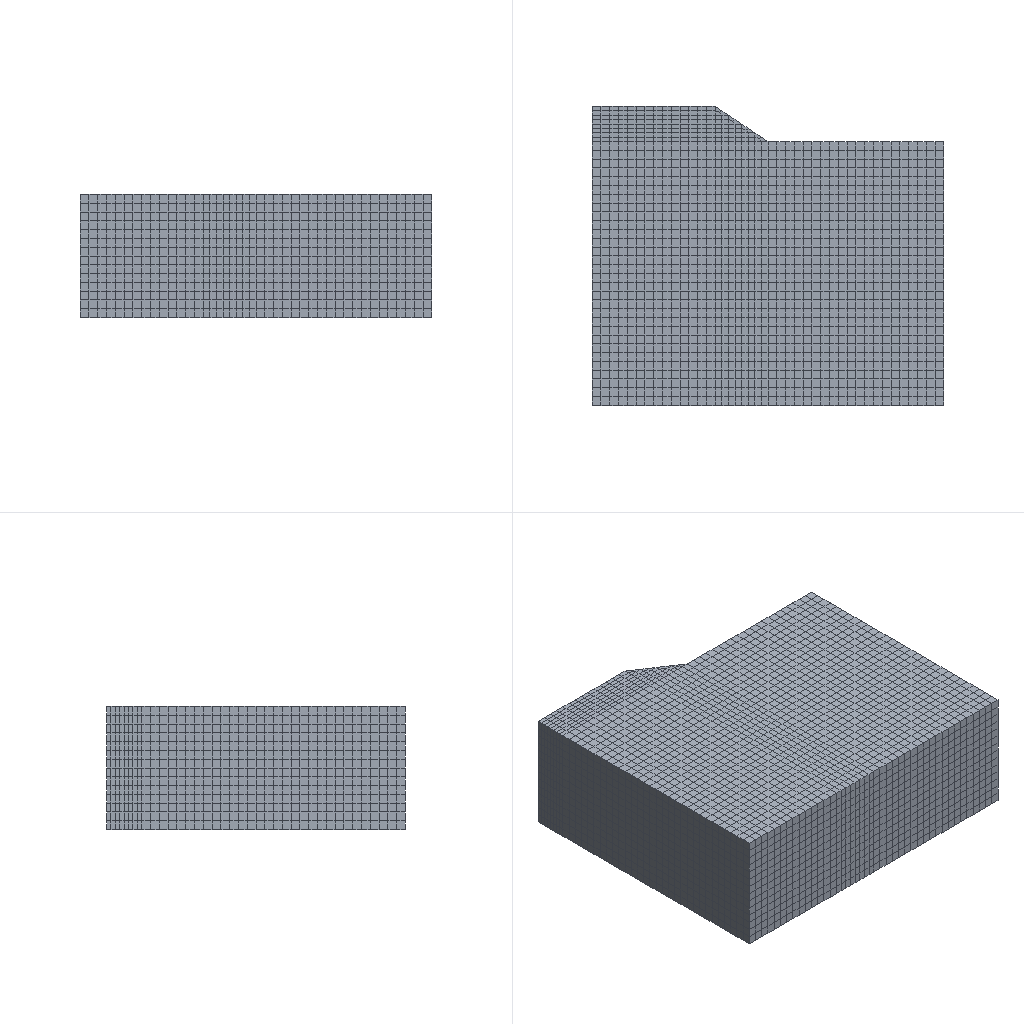Simulation study | abaqus
Set-up summary:
category,name,step,type,value,unit,region
solver,abaqus,,Abaqus/CAE 2024
units,SI m-kg-s (Pa),,inferred,E=3.71e+08 density=1800
analysis,Gravity,,geostatic,time_period=1
mesh,nodes,,,22275
mesh,elements,,,19712
element_type,C3D8R,,,19712
material,soil,,E,3.71e+08
material,soil,,nu,0.3
material,soil,,density,1800
material,soil,,behaviors,plastic; mohr coulomb; mohr coulomb hardening
section,soil,,solid section,,,_PickedSet2_#1
section,soil,,solid section,,,_PickedSet2_#3
section,soil,,solid section,,,_PickedSet2_#4
section,soil,,solid section,,,_PickedSet2_#5
section,soil,,solid section,,,_PickedSet2_#6
section,soil,,solid section,,,_PickedSet2_#2
load,Load-2,Gravity,gravity,"9.8 [dir=(0, -1, 0)]",,whole model
bc,BC-1,initial,fixed,"[dofs=x,y,z n=3]",,_PickedSet33
bc,BC-2,initial,fixed,[dofs=x],,_PickedSet32
bc,BC-3,initial,fixed,[dofs=z],,_PickedSet31
Abaqus input file, long lists of numbers shortened:
*Heading
** Job name: deck Model name: Model-1-Copy
** Generated by: Abaqus/CAE 2024
*Preprint, echo=NO, model=NO, history=NO, contact=NO
**
** PARTS
**
*Part, name=Part-1
*Node
      1,          14.,          30.,           0.
      2,          14.,          30.,          14.
** (22273 more lines like these left out)
*Element, type=C3D8R
   1,  209, 1297, 6221,  891,    1,   39,  748,   66
   2, 1297, 1298, 6222, 6221,   39,   40,  749,  748
** (19710 more lines like these left out)
*Nset, nset=_PickedSet2_#1, internal
     1,     2,     3,     4,     5,     6,     7,     8,     9,    10,    11,    12,    13,    14,    15,    16
    17,    18,    19,    20,    21,    22,    39,    40,    41,    42,    43,    44,    45,    46,    47,    48
** (1248 more lines like these left out)
*Elset, elset=_PickedSet2_#1, internal, generate
     1,  17640,      1
*Nset, nset=_PickedSet2_#3, internal
     7,     8,     9,    10,    23,    24,    83,    84,    85,    86,    87,    88,    89,    90,    91,    92
    93,    94,    95,    97,    98,    99,   100,   101,   102,   103,   104,   105,   106,   107,   108,   109
** (5 more lines like these left out)
*Elset, elset=_PickedSet2_#3, internal, generate
 17641,  17682,      1
*Nset, nset=_PickedSet2_#4, internal
    23,    24,    25,    26,    27,    28,   566,   567,   568,   569,   570,   571,   572,   573,   574,   575
   576,   577,   578,   581,   582,   583,   584,   585,   586,   587,   588,   589,   590,   591,   592,   593
** (5 more lines like these left out)
*Elset, elset=_PickedSet2_#4, internal, generate
 17683,  17724,      1
*Nset, nset=_PickedSet2_#5, internal
    25,    26,    29,    30,    31,    32,   581,   582,   583,   584,   585,   586,   587,   588,   589,   590
   591,   592,   593,   613,   614,   615,   616,   617,   618,   619,   620,   621,   622,   623,   624,   625
** (5 more lines like these left out)
*Elset, elset=_PickedSet2_#5, internal, generate
 17725,  17766,      1
*Nset, nset=_PickedSet2_#6, internal
    29,    30,    33,    34,    35,    36,   613,   614,   615,   616,   617,   618,   619,   620,   621,   622
   623,   624,   625,   645,   646,   647,   648,   649,   650,   651,   652,   653,   654,   655,   656,   657
** (5 more lines like these left out)
*Elset, elset=_PickedSet2_#6, internal, generate
 17767,  17808,      1
*Nset, nset=_PickedSet2_#2, internal
     1,     2,     3,     4,     5,     6,     7,     8,    21,    22,    23,    24,    25,    26,    27,    28
    29,    30,    31,    32,    33,    34,    35,    36,    37,    38,    39,    40,    41,    42,    43,    44
** (153 more lines like these left out)
*Elset, elset=_PickedSet2_#2, internal, generate
 17809,  19712,      1
** Section: Section-1
*Solid Section, elset=_PickedSet2_#1, material=soil
,
** Section: Section-1
*Solid Section, elset=_PickedSet2_#3, material=soil
,
** Section: Section-1
*Solid Section, elset=_PickedSet2_#4, material=soil
,
** Section: Section-1
*Solid Section, elset=_PickedSet2_#5, material=soil
,
** Section: Section-1
*Solid Section, elset=_PickedSet2_#6, material=soil
,
** Section: Section-1
*Solid Section, elset=_PickedSet2_#2, material=soil
,
*End Part
**
**
** ASSEMBLY
**
*Assembly, name=Assembly
**
*Instance, name=Part-1-1, part=Part-1
*End Instance
**
*Nset, nset=Set-1, instance=Part-1-1
   29,   30,   33,   34,  613,  614,  615,  616,  617,  618,  619,  620,  621,  622,  623,  624
  625,  645,  646,  647,  648,  649,  650,  651,  652,  653,  654,  655,  656,  657,  658,  661
** (1 more lines like these left out)
*Elset, elset=Set-1, instance=Part-1-1, generate
 17767,  17794,      1
*Nset, nset=_PickedSet22, internal, instance=Part-1-1, generate
     1,  22275,      1
*Elset, elset=_PickedSet22, internal, instance=Part-1-1, generate
     1,  19712,      1
*Nset, nset=_PickedSet31, internal, instance=Part-1-1
    1,    2,    3,    4,    5,    6,    7,    8,    9,   10,   11,   12,   13,   14,   15,   16
   17,   18,   19,   20,   21,   22,   23,   24,   25,   26,   27,   28,   29,   30,   31,   32
** (184 more lines like these left out)
*Elset, elset=_PickedSet31, internal, instance=Part-1-1
     1,    14,    15,    28,    29,    42,    43,    56,    57,    70,    71,    84,    85,    98,    99,   112
   113,   126,   127,   140,   141,   154,   155,   168,   169,   182,   183,   196,   197,   210,   211,   224
** (174 more lines like these left out)
*Nset, nset=_PickedSet32, internal, instance=Part-1-1
   15,   16,   17,   18,   19,   20,   21,   22,   37,   38,  287,  288,  289,  290,  291,  292
  293,  294,  295,  296,  297,  298,  299,  338,  339,  340,  341,  342,  343,  344,  345,  346
** (64 more lines like these left out)
*Elset, elset=_PickedSet32, internal, instance=Part-1-1
  3627,  3628,  3629,  3630,  3631,  3632,  3633,  3634,  3635,  3636,  3637,  3638,  3639,  3640,  3907,  3908
  3909,  3910,  3911,  3912,  3913,  3914,  3915,  3916,  3917,  3918,  3919,  3920,  4187,  4188,  4189,  4190
** (58 more lines like these left out)
*Nset, nset=_PickedSet33, internal, instance=Part-1-1
   11,   12,   13,   14,   17,   18,   19,   20,  112,  113,  114,  115,  116,  117,  118,  119
  120,  121,  122,  123,  124,  125,  126,  127,  128,  129,  130,  131,  132,  133,  134,  135
** (39 more lines like these left out)
*Elset, elset=_PickedSet33, internal, instance=Part-1-1
  3249,  3250,  3251,  3252,  3253,  3254,  3255,  3256,  3257,  3258,  3259,  3260,  3261,  3262,  3263,  3264
  3265,  3266,  3267,  3268,  3269,  3270,  3271,  3272,  3273,  3274,  3275,  3276,  3277,  3278,  3279,  3280
** (35 more lines like these left out)
*Elset, elset=_Surf-1_S2, internal, instance=Part-1-1
    1,    2,    3,    4,    5,    6,    7,    8,    9,   10,   11,   12,   13,   14,   15,   16
   17,   18,   19,   20,   21,   22,   23,   24,   25,   26,   27,   28,   29,   30,   31,   32
** (23 more lines like these left out)
*Elset, elset=_Surf-1_S1, internal, instance=Part-1-1, generate
 17445,  17640,      1
*Surface, type=ELEMENT, name=Surf-1
_Surf-1_S2, S2
_Surf-1_S1, S1
*Elset, elset=_Surf-2_S2, internal, instance=Part-1-1, generate
   1,  112,    1
*Elset, elset=_Surf-2_S1, internal, instance=Part-1-1, generate
 17445,  17640,      1
*Surface, type=ELEMENT, name=Surf-2
_Surf-2_S2, S2
_Surf-2_S1, S1
*Elset, elset=_Surf-3_S2, internal, instance=Part-1-1
    85,    86,    87,    88,    89,    90,    91,    92,    93,    94,    95,    96,    97,    98,    99,   100
   101,   102,   103,   104,   105,   106,   107,   108,   109,   110,   111,   112, 17718, 17719, 17720, 17721
** (2 more lines like these left out)
*Elset, elset=_Surf-3_S4, internal, instance=Part-1-1
 17648, 17649, 17650, 17651, 17652, 17653, 17654, 17669, 17670, 17671, 17672, 17673, 17674, 17675, 17690, 17691
 17692, 17693, 17694, 17695, 17696, 17704, 17705, 17706, 17707, 17708, 17709, 17710, 17711, 17712, 17713, 17714
** (5 more lines like these left out)
*Elset, elset=_Surf-3_S3, internal, instance=Part-1-1
 17655, 17656, 17657, 17658, 17659, 17660, 17661, 17676, 17677, 17678, 17679, 17680, 17681, 17682, 17683, 17684
 17685, 17686, 17687, 17688, 17689, 17697, 17698, 17699, 17700, 17701, 17702, 17703, 17711, 17712, 17713, 17714
** (3 more lines like these left out)
*Surface, type=ELEMENT, name=Surf-3
_Surf-3_S2, S2
_Surf-3_S4, S4
_Surf-3_S3, S3
*Elset, elset=_Surf-4_S4, internal, instance=Part-1-1
 17648, 17649, 17650, 17651, 17652, 17653, 17654, 17669, 17670, 17671, 17672, 17673, 17674, 17675, 17690, 17691
 17692, 17693, 17694, 17695, 17696, 17704, 17705, 17706, 17707, 17708, 17709, 17710, 17711, 17712, 17713, 17714
** (5 more lines like these left out)
*Elset, elset=_Surf-4_S3, internal, instance=Part-1-1
 17655, 17656, 17657, 17658, 17659, 17660, 17661, 17676, 17677, 17678, 17679, 17680, 17681, 17682, 17683, 17684
 17685, 17686, 17687, 17688, 17689, 17697, 17698, 17699, 17700, 17701, 17702, 17703, 17711, 17712, 17713, 17714
** (3 more lines like these left out)
*Elset, elset=_Surf-4_S2, internal, instance=Part-1-1
 17718, 17719, 17720, 17721, 17722, 17723, 17724, 17760, 17761, 17762, 17763, 17764, 17765, 17766, 17802, 17803
 17804, 17805, 17806, 17807, 17808
*Surface, type=ELEMENT, name=Surf-4
_Surf-4_S4, S4
_Surf-4_S3, S3
_Surf-4_S2, S2
*End Assembly
**
** MATERIALS
**
*Material, name=soil
*Density
1800.,
*Elastic
 3.71e+08, 0.3
*Mohr Coulomb
30., 0.1
*Mohr Coulomb Hardening
100000.,0.
**
** INTERACTION PROPERTIES
**
*Surface Interaction, name=IntProp-1
1.,
*Friction
0.,
*Surface Behavior, pressure-overclosure=HARD
**
** BOUNDARY CONDITIONS
**
** Name: BC-1 Type: Displacement/Rotation
*Boundary
_PickedSet33, 1, 1
_PickedSet33, 2, 2
_PickedSet33, 3, 3
** Name: BC-2 Type: Displacement/Rotation
*Boundary
_PickedSet32, 1, 1
** Name: BC-3 Type: Displacement/Rotation
*Boundary
_PickedSet31, 3, 3
** ----------------------------------------------------------------
**
** STEP: Gravity
**
*Step, name=Gravity, nlgeom=NO
*Geostatic, utol=1.
0.1, 1., 1e-05, 0.1
**
** LOADS
**
** Name: Load-2   Type: Gravity
*Dload
, GRAV, 9.8, 0., -1., 0.
**
** OUTPUT REQUESTS
**
*Restart, write, frequency=0
**
** FIELD OUTPUT: F-Output-1
**
*Output, field, variable=PRESELECT
**
** HISTORY OUTPUT: H-Output-1
**
*Output, history, variable=PRESELECT
*End Step
Results summary:
result,odb.job_status,,,JOB_STATUS_COMPLETED_SUCCESSFULLY,"consistent, unstated (Abaqus has no unit system)"
result,steps[0].procedure,Gravity,,*GEOSTATIC,"consistent, unstated (Abaqus has no unit system)"
result,steps[0].time_period,Gravity,,1,"consistent, unstated (Abaqus has no unit system)"
result,steps[0].n_frames,Gravity,,11,"consistent, unstated (Abaqus has no unit system)"
result,steps[0].last_frame.id,Gravity,,10,"consistent, unstated (Abaqus has no unit system)"
result,steps[0].last_frame.value,Gravity,,1,"consistent, unstated (Abaqus has no unit system)"
result,steps[0].last_frame.description,Gravity,,Increment     10: Step Time =    1.000,"consistent, unstated (Abaqus has no unit system)"
result,steps[0].completed,Gravity,,True,"consistent, unstated (Abaqus has no unit system)"
result,steps[0].max_U_magnitude,Gravity,,0.02015,"consistent, unstated (Abaqus has no unit system)"
result,steps[0].max_S_mises,Gravity,,326533,"consistent, unstated (Abaqus has no unit system)"
result,steps[0].RF_sum[1],Gravity,,-2.057,"consistent, unstated (Abaqus has no unit system)"
result,steps[0].RF_sum[2],Gravity,,3.13145e+08,"consistent, unstated (Abaqus has no unit system)"
result,steps[0].RF_sum[3],Gravity,,-78.738,"consistent, unstated (Abaqus has no unit system)"